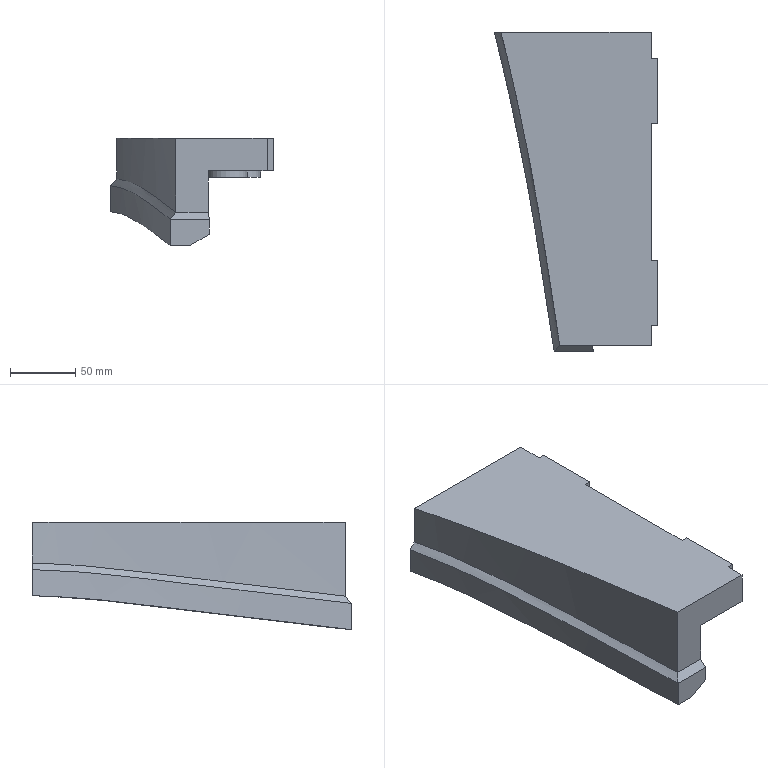Part | NX | features solid 2 | 1 solid | 31 faces | box 125.127 x 245 x 82.32 mm | volume 850947 mm3 | plane 20 | spline 6 | cylinder 5 | commonest cylinder face diameters 30 x5